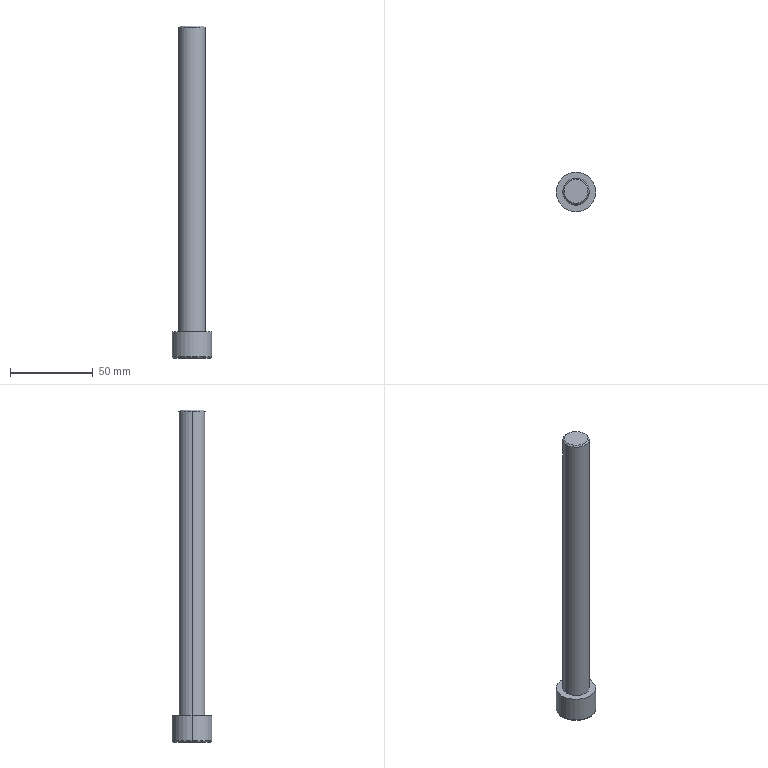Part | Creo | 1 solid | 20 faces | box 24 x 24 x 201 mm | volume 43051 mm3 | plane 10 | cylinder 4 | torus 4 | cone 2 | commonest cylinder face diameters 16 x2 24 x2
STEP:
#1=CARTESIAN_POINT('',(0.,0.,0.));
#2=DIRECTION('',(0.,0.,1.));
#3=DIRECTION('',(1.,0.,0.));
#4=AXIS2_PLACEMENT_3D('',#1,#2,#3);
#5=CARTESIAN_POINT('',(-153.,0.,-293.2));
#6=VERTEX_POINT('',#5);
#7=CARTESIAN_POINT('',(-177.,0.,-293.2));
#8=VERTEX_POINT('',#7);
#9=CARTESIAN_POINT('',(-165.,0.,-293.2));
#10=DIRECTION('',(0.,0.,-1.));
#11=DIRECTION('',(1.,0.,0.));
#12=AXIS2_PLACEMENT_3D('',#9,#10,#11);
#13=CIRCLE('',#12,12.);
#14=EDGE_CURVE('',#6,#8,#13,.T.);
#15=ORIENTED_EDGE('',*,*,#14,.T.);
#16=CARTESIAN_POINT('',(-177.,0.,-278.));
#17=VERTEX_POINT('',#16);
#18=CARTESIAN_POINT('',(-177.,0.,-278.));
#19=DIRECTION('',(0.,0.,-1.));
#20=VECTOR('',#19,15.2);
#21=LINE('',#18,#20);
#22=EDGE_CURVE('',#17,#8,#21,.T.);
#23=ORIENTED_EDGE('',*,*,#22,.F.);
#24=CARTESIAN_POINT('',(-153.,0.,-278.));
#25=VERTEX_POINT('',#24);
#26=CARTESIAN_POINT('',(-165.,0.,-278.));
#27=DIRECTION('',(0.,0.,1.));
#28=DIRECTION('',(-1.,0.,0.));
#29=AXIS2_PLACEMENT_3D('',#26,#27,#28);
#30=CIRCLE('',#29,12.);
#31=EDGE_CURVE('',#17,#25,#30,.T.);
#32=ORIENTED_EDGE('',*,*,#31,.T.);
#33=CARTESIAN_POINT('',(-153.,0.,-278.));
#34=DIRECTION('',(0.,0.,-1.));
#35=VECTOR('',#34,15.2);
#36=LINE('',#33,#35);
#37=EDGE_CURVE('',#25,#6,#36,.T.);
#38=ORIENTED_EDGE('',*,*,#37,.T.);
#39=EDGE_LOOP('',(#15,#23,#32,#38));
#40=FACE_OUTER_BOUND('',#39,.F.);
#41=CARTESIAN_POINT('',(-165.,0.,-278.));
#42=DIRECTION('',(0.,0.,-1.));
#43=DIRECTION('',(1.,0.,0.));
#44=AXIS2_PLACEMENT_3D('',#41,#42,#43);
#45=CYLINDRICAL_SURFACE('',#44,12.);
#46=ADVANCED_FACE('',(#40),#45,.T.);
#47=ORIENTED_EDGE('',*,*,#14,.F.);
#48=CARTESIAN_POINT('',(-153.234,0.,-293.766));
#49=VERTEX_POINT('',#48);
#50=CARTESIAN_POINT('',(-153.8,0.,-293.2));
#51=DIRECTION('',(0.,1.,0.));
#52=DIRECTION('',(1.,0.,0.));
#53=AXIS2_PLACEMENT_3D('',#50,#51,#52);
#54=CIRCLE('',#53,0.8);
#55=EDGE_CURVE('',#6,#49,#54,.T.);
#56=ORIENTED_EDGE('',*,*,#55,.T.);
#57=CARTESIAN_POINT('',(-176.766,0.,-293.766));
#58=VERTEX_POINT('',#57);
#59=CARTESIAN_POINT('',(-165.,0.,-293.766));
#60=DIRECTION('',(0.,0.,-1.));
#61=DIRECTION('',(1.,0.,0.));
#62=AXIS2_PLACEMENT_3D('',#59,#60,#61);
#63=CIRCLE('',#62,11.766);
#64=EDGE_CURVE('',#49,#58,#63,.T.);
#65=ORIENTED_EDGE('',*,*,#64,.T.);
#66=CARTESIAN_POINT('',(-176.2,0.,-293.2));
#67=DIRECTION('',(0.,-1.,0.));
#68=DIRECTION('',(-1.,0.,0.));
#69=AXIS2_PLACEMENT_3D('',#66,#67,#68);
#70=CIRCLE('',#69,0.8);
#71=EDGE_CURVE('',#8,#58,#70,.T.);
#72=ORIENTED_EDGE('',*,*,#71,.F.);
#73=EDGE_LOOP('',(#47,#56,#65,#72));
#74=FACE_OUTER_BOUND('',#73,.F.);
#75=CARTESIAN_POINT('',(-165.,0.,-293.2));
#76=DIRECTION('',(0.,0.,-1.));
#77=DIRECTION('',(1.,0.,0.));
#78=AXIS2_PLACEMENT_3D('',#75,#76,#77);
#79=TOROIDAL_SURFACE('',#78,11.2,0.8);
#80=ADVANCED_FACE('',(#74),#79,.T.);
#81=CARTESIAN_POINT('',(-165.,0.,-293.2));
#82=DIRECTION('',(0.,0.,-1.));
#83=DIRECTION('',(-1.,0.,0.));
#84=AXIS2_PLACEMENT_3D('',#81,#82,#83);
#85=CIRCLE('',#84,12.);
#86=EDGE_CURVE('',#8,#6,#85,.T.);
#87=ORIENTED_EDGE('',*,*,#86,.F.);
#88=ORIENTED_EDGE('',*,*,#71,.T.);
#89=CARTESIAN_POINT('',(-165.,0.,-293.766));
#90=DIRECTION('',(0.,0.,-1.));
#91=DIRECTION('',(-1.,0.,0.));
#92=AXIS2_PLACEMENT_3D('',#89,#90,#91);
#93=CIRCLE('',#92,11.766);
#94=EDGE_CURVE('',#58,#49,#93,.T.);
#95=ORIENTED_EDGE('',*,*,#94,.T.);
#96=ORIENTED_EDGE('',*,*,#55,.F.);
#97=EDGE_LOOP('',(#87,#88,#95,#96));
#98=FACE_OUTER_BOUND('',#97,.F.);
#99=CARTESIAN_POINT('',(-165.,0.,-293.2));
#100=DIRECTION('',(0.,0.,-1.));
#101=DIRECTION('',(1.,0.,0.));
#102=AXIS2_PLACEMENT_3D('',#99,#100,#101);
#103=TOROIDAL_SURFACE('',#102,11.2,0.8);
#104=ADVANCED_FACE('',(#98),#103,.T.);
#105=ORIENTED_EDGE('',*,*,#86,.T.);
#106=ORIENTED_EDGE('',*,*,#37,.F.);
#107=CARTESIAN_POINT('',(-165.,0.,-278.));
#108=DIRECTION('',(0.,0.,1.));
#109=DIRECTION('',(1.,0.,0.));
#110=AXIS2_PLACEMENT_3D('',#107,#108,#109);
#111=CIRCLE('',#110,12.);
#112=EDGE_CURVE('',#25,#17,#111,.T.);
#113=ORIENTED_EDGE('',*,*,#112,.T.);
#114=ORIENTED_EDGE('',*,*,#22,.T.);
#115=EDGE_LOOP('',(#105,#106,#113,#114));
#116=FACE_OUTER_BOUND('',#115,.F.);
#117=CARTESIAN_POINT('',(-165.,0.,-278.));
#118=DIRECTION('',(0.,0.,-1.));
#119=DIRECTION('',(1.,0.,0.));
#120=AXIS2_PLACEMENT_3D('',#117,#118,#119);
#121=CYLINDRICAL_SURFACE('',#120,12.);
#122=ADVANCED_FACE('',(#116),#121,.T.);
#123=ORIENTED_EDGE('',*,*,#31,.F.);
#124=ORIENTED_EDGE('',*,*,#112,.F.);
#125=EDGE_LOOP('',(#123,#124));
#126=FACE_OUTER_BOUND('',#125,.F.);
#127=CARTESIAN_POINT('',(-157.,0.,-278.));
#128=VERTEX_POINT('',#127);
#129=CARTESIAN_POINT('',(-173.,0.,-278.));
#130=VERTEX_POINT('',#129);
#131=CARTESIAN_POINT('',(-165.,0.,-278.));
#132=DIRECTION('',(0.,0.,-1.));
#133=DIRECTION('',(1.,0.,0.));
#134=AXIS2_PLACEMENT_3D('',#131,#132,#133);
#135=CIRCLE('',#134,8.);
#136=EDGE_CURVE('',#128,#130,#135,.T.);
#137=ORIENTED_EDGE('',*,*,#136,.F.);
#138=CARTESIAN_POINT('',(-165.,0.,-278.));
#139=DIRECTION('',(0.,0.,-1.));
#140=DIRECTION('',(-1.,0.,0.));
#141=AXIS2_PLACEMENT_3D('',#138,#139,#140);
#142=CIRCLE('',#141,8.);
#143=EDGE_CURVE('',#130,#128,#142,.T.);
#144=ORIENTED_EDGE('',*,*,#143,.F.);
#145=EDGE_LOOP('',(#137,#144));
#146=FACE_BOUND('',#145,.F.);
#147=CARTESIAN_POINT('',(-165.,0.,-278.));
#148=DIRECTION('',(0.,0.,-1.));
#149=DIRECTION('',(1.,0.,0.));
#150=AXIS2_PLACEMENT_3D('',#147,#148,#149);
#151=PLANE('',#150);
#152=ADVANCED_FACE('',(#126,#146),#151,.F.);
#153=CARTESIAN_POINT('',(-173.,0.,-93.8));
#154=VERTEX_POINT('',#153);
#155=CARTESIAN_POINT('',(-157.,0.,-93.8));
#156=VERTEX_POINT('',#155);
#157=CARTESIAN_POINT('',(-165.,0.,-93.8));
#158=DIRECTION('',(0.,0.,1.));
#159=DIRECTION('',(-1.,0.,0.));
#160=AXIS2_PLACEMENT_3D('',#157,#158,#159);
#161=CIRCLE('',#160,8.);
#162=EDGE_CURVE('',#154,#156,#161,.T.);
#163=ORIENTED_EDGE('',*,*,#162,.T.);
#164=CARTESIAN_POINT('',(-157.,0.,-278.));
#165=DIRECTION('',(0.,0.,1.));
#166=VECTOR('',#165,184.2);
#167=LINE('',#164,#166);
#168=EDGE_CURVE('',#128,#156,#167,.T.);
#169=ORIENTED_EDGE('',*,*,#168,.F.);
#170=ORIENTED_EDGE('',*,*,#136,.T.);
#171=CARTESIAN_POINT('',(-173.,0.,-278.));
#172=DIRECTION('',(0.,0.,1.));
#173=VECTOR('',#172,184.2);
#174=LINE('',#171,#173);
#175=EDGE_CURVE('',#130,#154,#174,.T.);
#176=ORIENTED_EDGE('',*,*,#175,.T.);
#177=EDGE_LOOP('',(#163,#169,#170,#176));
#178=FACE_OUTER_BOUND('',#177,.F.);
#179=CARTESIAN_POINT('',(-165.,0.,-278.));
#180=DIRECTION('',(0.,0.,1.));
#181=DIRECTION('',(-1.,0.,0.));
#182=AXIS2_PLACEMENT_3D('',#179,#180,#181);
#183=CYLINDRICAL_SURFACE('',#182,8.);
#184=ADVANCED_FACE('',(#178),#183,.T.);
#185=ORIENTED_EDGE('',*,*,#162,.F.);
#186=CARTESIAN_POINT('',(-172.2,0.,-93.));
#187=VERTEX_POINT('',#186);
#188=CARTESIAN_POINT('',(-172.2,0.,-93.));
#189=DIRECTION('',(-0.7071,0.,-0.7071));
#190=VECTOR('',#189,1.131);
#191=LINE('',#188,#190);
#192=EDGE_CURVE('',#187,#154,#191,.T.);
#193=ORIENTED_EDGE('',*,*,#192,.F.);
#194=CARTESIAN_POINT('',(-157.8,0.,-93.));
#195=VERTEX_POINT('',#194);
#196=CARTESIAN_POINT('',(-165.,0.,-93.));
#197=DIRECTION('',(0.,0.,1.));
#198=DIRECTION('',(-1.,0.,0.));
#199=AXIS2_PLACEMENT_3D('',#196,#197,#198);
#200=CIRCLE('',#199,7.2);
#201=EDGE_CURVE('',#187,#195,#200,.T.);
#202=ORIENTED_EDGE('',*,*,#201,.T.);
#203=CARTESIAN_POINT('',(-157.8,0.,-93.));
#204=DIRECTION('',(0.7071,0.,-0.7071));
#205=VECTOR('',#204,1.131);
#206=LINE('',#203,#205);
#207=EDGE_CURVE('',#195,#156,#206,.T.);
#208=ORIENTED_EDGE('',*,*,#207,.T.);
#209=EDGE_LOOP('',(#185,#193,#202,#208));
#210=FACE_OUTER_BOUND('',#209,.F.);
#211=CARTESIAN_POINT('',(-165.,0.,-93.4));
#212=DIRECTION('',(0.,0.,-1.));
#213=DIRECTION('',(1.,0.,0.));
#214=AXIS2_PLACEMENT_3D('',#211,#212,#213);
#215=CONICAL_SURFACE('',#214,7.6,45.);
#216=ADVANCED_FACE('',(#210),#215,.T.);
#217=CARTESIAN_POINT('',(-165.,0.,-93.8));
#218=DIRECTION('',(0.,0.,1.));
#219=DIRECTION('',(1.,0.,0.));
#220=AXIS2_PLACEMENT_3D('',#217,#218,#219);
#221=CIRCLE('',#220,8.);
#222=EDGE_CURVE('',#156,#154,#221,.T.);
#223=ORIENTED_EDGE('',*,*,#222,.F.);
#224=ORIENTED_EDGE('',*,*,#207,.F.);
#225=CARTESIAN_POINT('',(-165.,0.,-93.));
#226=DIRECTION('',(0.,0.,1.));
#227=DIRECTION('',(1.,0.,0.));
#228=AXIS2_PLACEMENT_3D('',#225,#226,#227);
#229=CIRCLE('',#228,7.2);
#230=EDGE_CURVE('',#195,#187,#229,.T.);
#231=ORIENTED_EDGE('',*,*,#230,.T.);
#232=ORIENTED_EDGE('',*,*,#192,.T.);
#233=EDGE_LOOP('',(#223,#224,#231,#232));
#234=FACE_OUTER_BOUND('',#233,.F.);
#235=CARTESIAN_POINT('',(-165.,0.,-93.4));
#236=DIRECTION('',(0.,0.,-1.));
#237=DIRECTION('',(1.,0.,0.));
#238=AXIS2_PLACEMENT_3D('',#235,#236,#237);
#239=CONICAL_SURFACE('',#238,7.6,45.);
#240=ADVANCED_FACE('',(#234),#239,.T.);
#241=ORIENTED_EDGE('',*,*,#222,.T.);
#242=ORIENTED_EDGE('',*,*,#175,.F.);
#243=ORIENTED_EDGE('',*,*,#143,.T.);
#244=ORIENTED_EDGE('',*,*,#168,.T.);
#245=EDGE_LOOP('',(#241,#242,#243,#244));
#246=FACE_OUTER_BOUND('',#245,.F.);
#247=CARTESIAN_POINT('',(-165.,0.,-278.));
#248=DIRECTION('',(0.,0.,1.));
#249=DIRECTION('',(-1.,0.,0.));
#250=AXIS2_PLACEMENT_3D('',#247,#248,#249);
#251=CYLINDRICAL_SURFACE('',#250,8.);
#252=ADVANCED_FACE('',(#246),#251,.T.);
#253=ORIENTED_EDGE('',*,*,#230,.F.);
#254=ORIENTED_EDGE('',*,*,#201,.F.);
#255=EDGE_LOOP('',(#253,#254));
#256=FACE_OUTER_BOUND('',#255,.F.);
#257=CARTESIAN_POINT('',(-165.,0.,-93.));
#258=DIRECTION('',(0.,0.,1.));
#259=DIRECTION('',(-1.,0.,0.));
#260=AXIS2_PLACEMENT_3D('',#257,#258,#259);
#261=PLANE('',#260);
#262=ADVANCED_FACE('',(#256),#261,.T.);
#263=CARTESIAN_POINT('',(-176.2,0.,-294.));
#264=VERTEX_POINT('',#263);
#265=CARTESIAN_POINT('',(-153.8,0.,-294.));
#266=VERTEX_POINT('',#265);
#267=CARTESIAN_POINT('',(-165.,0.,-294.));
#268=DIRECTION('',(0.,0.,-1.));
#269=DIRECTION('',(-1.,0.,0.));
#270=AXIS2_PLACEMENT_3D('',#267,#268,#269);
#271=CIRCLE('',#270,11.2);
#272=EDGE_CURVE('',#264,#266,#271,.T.);
#273=ORIENTED_EDGE('',*,*,#272,.T.);
#274=CARTESIAN_POINT('',(-153.8,0.,-293.2));
#275=DIRECTION('',(0.,1.,0.));
#276=DIRECTION('',(0.7071,0.,-0.7071));
#277=AXIS2_PLACEMENT_3D('',#274,#275,#276);
#278=CIRCLE('',#277,0.8);
#279=EDGE_CURVE('',#49,#266,#278,.T.);
#280=ORIENTED_EDGE('',*,*,#279,.F.);
#281=ORIENTED_EDGE('',*,*,#94,.F.);
#282=CARTESIAN_POINT('',(-176.2,0.,-293.2));
#283=DIRECTION('',(0.,-1.,0.));
#284=DIRECTION('',(-0.7071,0.,-0.7071));
#285=AXIS2_PLACEMENT_3D('',#282,#283,#284);
#286=CIRCLE('',#285,0.8);
#287=EDGE_CURVE('',#58,#264,#286,.T.);
#288=ORIENTED_EDGE('',*,*,#287,.T.);
#289=EDGE_LOOP('',(#273,#280,#281,#288));
#290=FACE_OUTER_BOUND('',#289,.F.);
#291=CARTESIAN_POINT('',(-165.,0.,-293.2));
#292=DIRECTION('',(0.,0.,-1.));
#293=DIRECTION('',(1.,0.,0.));
#294=AXIS2_PLACEMENT_3D('',#291,#292,#293);
#295=TOROIDAL_SURFACE('',#294,11.2,0.8);
#296=ADVANCED_FACE('',(#290),#295,.T.);
#297=ORIENTED_EDGE('',*,*,#272,.F.);
#298=CARTESIAN_POINT('',(-165.,0.,-294.));
#299=DIRECTION('',(0.,0.,-1.));
#300=DIRECTION('',(1.,0.,0.));
#301=AXIS2_PLACEMENT_3D('',#298,#299,#300);
#302=CIRCLE('',#301,11.2);
#303=EDGE_CURVE('',#266,#264,#302,.T.);
#304=ORIENTED_EDGE('',*,*,#303,.F.);
#305=EDGE_LOOP('',(#297,#304));
#306=FACE_OUTER_BOUND('',#305,.F.);
#307=CARTESIAN_POINT('',(-169.041,-7.,-294.));
#308=VERTEX_POINT('',#307);
#309=CARTESIAN_POINT('',(-160.959,-7.,-294.));
#310=VERTEX_POINT('',#309);
#311=CARTESIAN_POINT('',(-169.041,-7.,-294.));
#312=DIRECTION('',(1.,0.,0.));
#313=VECTOR('',#312,8.083);
#314=LINE('',#311,#313);
#315=EDGE_CURVE('',#308,#310,#314,.T.);
#316=ORIENTED_EDGE('',*,*,#315,.F.);
#317=CARTESIAN_POINT('',(-173.083,0.,-294.));
#318=VERTEX_POINT('',#317);
#319=CARTESIAN_POINT('',(-173.083,0.,-294.));
#320=DIRECTION('',(0.5,-0.866,0.));
#321=VECTOR('',#320,8.083);
#322=LINE('',#319,#321);
#323=EDGE_CURVE('',#318,#308,#322,.T.);
#324=ORIENTED_EDGE('',*,*,#323,.F.);
#325=CARTESIAN_POINT('',(-169.041,7.,-294.));
#326=VERTEX_POINT('',#325);
#327=CARTESIAN_POINT('',(-169.041,7.,-294.));
#328=DIRECTION('',(-0.5,-0.866,0.));
#329=VECTOR('',#328,8.083);
#330=LINE('',#327,#329);
#331=EDGE_CURVE('',#326,#318,#330,.T.);
#332=ORIENTED_EDGE('',*,*,#331,.F.);
#333=CARTESIAN_POINT('',(-160.959,7.,-294.));
#334=VERTEX_POINT('',#333);
#335=CARTESIAN_POINT('',(-160.959,7.,-294.));
#336=DIRECTION('',(-1.,0.,0.));
#337=VECTOR('',#336,8.083);
#338=LINE('',#335,#337);
#339=EDGE_CURVE('',#334,#326,#338,.T.);
#340=ORIENTED_EDGE('',*,*,#339,.F.);
#341=CARTESIAN_POINT('',(-156.917,0.,-294.));
#342=VERTEX_POINT('',#341);
#343=CARTESIAN_POINT('',(-156.917,0.,-294.));
#344=DIRECTION('',(-0.5,0.866,0.));
#345=VECTOR('',#344,8.083);
#346=LINE('',#343,#345);
#347=EDGE_CURVE('',#342,#334,#346,.T.);
#348=ORIENTED_EDGE('',*,*,#347,.F.);
#349=CARTESIAN_POINT('',(-160.959,-7.,-294.));
#350=DIRECTION('',(0.5,0.866,0.));
#351=VECTOR('',#350,8.083);
#352=LINE('',#349,#351);
#353=EDGE_CURVE('',#310,#342,#352,.T.);
#354=ORIENTED_EDGE('',*,*,#353,.F.);
#355=EDGE_LOOP('',(#316,#324,#332,#340,#348,#354));
#356=FACE_BOUND('',#355,.F.);
#357=CARTESIAN_POINT('',(-165.,0.,-294.));
#358=DIRECTION('',(0.,0.,-1.));
#359=DIRECTION('',(1.,0.,0.));
#360=AXIS2_PLACEMENT_3D('',#357,#358,#359);
#361=PLANE('',#360);
#362=ADVANCED_FACE('',(#306,#356),#361,.T.);
#363=ORIENTED_EDGE('',*,*,#303,.T.);
#364=ORIENTED_EDGE('',*,*,#287,.F.);
#365=ORIENTED_EDGE('',*,*,#64,.F.);
#366=ORIENTED_EDGE('',*,*,#279,.T.);
#367=EDGE_LOOP('',(#363,#364,#365,#366));
#368=FACE_OUTER_BOUND('',#367,.F.);
#369=CARTESIAN_POINT('',(-165.,0.,-293.2));
#370=DIRECTION('',(0.,0.,-1.));
#371=DIRECTION('',(1.,0.,0.));
#372=AXIS2_PLACEMENT_3D('',#369,#370,#371);
#373=TOROIDAL_SURFACE('',#372,11.2,0.8);
#374=ADVANCED_FACE('',(#368),#373,.T.);
#375=ORIENTED_EDGE('',*,*,#315,.T.);
#376=CARTESIAN_POINT('',(-160.959,-7.,-286.));
#377=VERTEX_POINT('',#376);
#378=CARTESIAN_POINT('',(-160.959,-7.,-294.));
#379=DIRECTION('',(0.,0.,1.));
#380=VECTOR('',#379,8.);
#381=LINE('',#378,#380);
#382=EDGE_CURVE('',#310,#377,#381,.T.);
#383=ORIENTED_EDGE('',*,*,#382,.T.);
#384=CARTESIAN_POINT('',(-169.041,-7.,-286.));
#385=VERTEX_POINT('',#384);
#386=CARTESIAN_POINT('',(-169.041,-7.,-286.));
#387=DIRECTION('',(1.,0.,0.));
#388=VECTOR('',#387,8.083);
#389=LINE('',#386,#388);
#390=EDGE_CURVE('',#385,#377,#389,.T.);
#391=ORIENTED_EDGE('',*,*,#390,.F.);
#392=CARTESIAN_POINT('',(-169.041,-7.,-294.));
#393=DIRECTION('',(0.,0.,1.));
#394=VECTOR('',#393,8.);
#395=LINE('',#392,#394);
#396=EDGE_CURVE('',#308,#385,#395,.T.);
#397=ORIENTED_EDGE('',*,*,#396,.F.);
#398=EDGE_LOOP('',(#375,#383,#391,#397));
#399=FACE_OUTER_BOUND('',#398,.F.);
#400=CARTESIAN_POINT('',(-160.959,-7.,-286.));
#401=DIRECTION('',(0.,-1.,0.));
#402=DIRECTION('',(1.,0.,0.));
#403=AXIS2_PLACEMENT_3D('',#400,#401,#402);
#404=PLANE('',#403);
#405=ADVANCED_FACE('',(#399),#404,.F.);
#406=ORIENTED_EDGE('',*,*,#353,.T.);
#407=CARTESIAN_POINT('',(-156.917,0.,-286.));
#408=VERTEX_POINT('',#407);
#409=CARTESIAN_POINT('',(-156.917,0.,-294.));
#410=DIRECTION('',(0.,0.,1.));
#411=VECTOR('',#410,8.);
#412=LINE('',#409,#411);
#413=EDGE_CURVE('',#342,#408,#412,.T.);
#414=ORIENTED_EDGE('',*,*,#413,.T.);
#415=CARTESIAN_POINT('',(-156.917,0.,-286.));
#416=DIRECTION('',(-0.5,-0.866,0.));
#417=VECTOR('',#416,8.083);
#418=LINE('',#415,#417);
#419=EDGE_CURVE('',#408,#377,#418,.T.);
#420=ORIENTED_EDGE('',*,*,#419,.T.);
#421=ORIENTED_EDGE('',*,*,#382,.F.);
#422=EDGE_LOOP('',(#406,#414,#420,#421));
#423=FACE_OUTER_BOUND('',#422,.F.);
#424=CARTESIAN_POINT('',(-156.917,0.,-286.));
#425=DIRECTION('',(0.866,-0.5,0.));
#426=DIRECTION('',(0.5,0.866,0.));
#427=AXIS2_PLACEMENT_3D('',#424,#425,#426);
#428=PLANE('',#427);
#429=ADVANCED_FACE('',(#423),#428,.F.);
#430=ORIENTED_EDGE('',*,*,#347,.T.);
#431=CARTESIAN_POINT('',(-160.959,7.,-286.));
#432=VERTEX_POINT('',#431);
#433=CARTESIAN_POINT('',(-160.959,7.,-294.));
#434=DIRECTION('',(0.,0.,1.));
#435=VECTOR('',#434,8.);
#436=LINE('',#433,#435);
#437=EDGE_CURVE('',#334,#432,#436,.T.);
#438=ORIENTED_EDGE('',*,*,#437,.T.);
#439=CARTESIAN_POINT('',(-160.959,7.,-286.));
#440=DIRECTION('',(0.5,-0.866,0.));
#441=VECTOR('',#440,8.083);
#442=LINE('',#439,#441);
#443=EDGE_CURVE('',#432,#408,#442,.T.);
#444=ORIENTED_EDGE('',*,*,#443,.T.);
#445=ORIENTED_EDGE('',*,*,#413,.F.);
#446=EDGE_LOOP('',(#430,#438,#444,#445));
#447=FACE_OUTER_BOUND('',#446,.F.);
#448=CARTESIAN_POINT('',(-160.959,7.,-286.));
#449=DIRECTION('',(0.866,0.5,0.));
#450=DIRECTION('',(-0.5,0.866,0.));
#451=AXIS2_PLACEMENT_3D('',#448,#449,#450);
#452=PLANE('',#451);
#453=ADVANCED_FACE('',(#447),#452,.F.);
#454=ORIENTED_EDGE('',*,*,#339,.T.);
#455=CARTESIAN_POINT('',(-169.041,7.,-286.));
#456=VERTEX_POINT('',#455);
#457=CARTESIAN_POINT('',(-169.041,7.,-294.));
#458=DIRECTION('',(0.,0.,1.));
#459=VECTOR('',#458,8.);
#460=LINE('',#457,#459);
#461=EDGE_CURVE('',#326,#456,#460,.T.);
#462=ORIENTED_EDGE('',*,*,#461,.T.);
#463=CARTESIAN_POINT('',(-160.959,7.,-286.));
#464=DIRECTION('',(-1.,0.,0.));
#465=VECTOR('',#464,8.083);
#466=LINE('',#463,#465);
#467=EDGE_CURVE('',#432,#456,#466,.T.);
#468=ORIENTED_EDGE('',*,*,#467,.F.);
#469=ORIENTED_EDGE('',*,*,#437,.F.);
#470=EDGE_LOOP('',(#454,#462,#468,#469));
#471=FACE_OUTER_BOUND('',#470,.F.);
#472=CARTESIAN_POINT('',(-169.041,7.,-286.));
#473=DIRECTION('',(0.,1.,0.));
#474=DIRECTION('',(-1.,0.,0.));
#475=AXIS2_PLACEMENT_3D('',#472,#473,#474);
#476=PLANE('',#475);
#477=ADVANCED_FACE('',(#471),#476,.F.);
#478=ORIENTED_EDGE('',*,*,#331,.T.);
#479=CARTESIAN_POINT('',(-173.083,0.,-286.));
#480=VERTEX_POINT('',#479);
#481=CARTESIAN_POINT('',(-173.083,0.,-294.));
#482=DIRECTION('',(0.,0.,1.));
#483=VECTOR('',#482,8.);
#484=LINE('',#481,#483);
#485=EDGE_CURVE('',#318,#480,#484,.T.);
#486=ORIENTED_EDGE('',*,*,#485,.T.);
#487=CARTESIAN_POINT('',(-173.083,0.,-286.));
#488=DIRECTION('',(0.5,0.866,0.));
#489=VECTOR('',#488,8.083);
#490=LINE('',#487,#489);
#491=EDGE_CURVE('',#480,#456,#490,.T.);
#492=ORIENTED_EDGE('',*,*,#491,.T.);
#493=ORIENTED_EDGE('',*,*,#461,.F.);
#494=EDGE_LOOP('',(#478,#486,#492,#493));
#495=FACE_OUTER_BOUND('',#494,.F.);
#496=CARTESIAN_POINT('',(-173.083,0.,-286.));
#497=DIRECTION('',(-0.866,0.5,0.));
#498=DIRECTION('',(-0.5,-0.866,0.));
#499=AXIS2_PLACEMENT_3D('',#496,#497,#498);
#500=PLANE('',#499);
#501=ADVANCED_FACE('',(#495),#500,.F.);
#502=ORIENTED_EDGE('',*,*,#323,.T.);
#503=ORIENTED_EDGE('',*,*,#396,.T.);
#504=CARTESIAN_POINT('',(-169.041,-7.,-286.));
#505=DIRECTION('',(-0.5,0.866,0.));
#506=VECTOR('',#505,8.083);
#507=LINE('',#504,#506);
#508=EDGE_CURVE('',#385,#480,#507,.T.);
#509=ORIENTED_EDGE('',*,*,#508,.T.);
#510=ORIENTED_EDGE('',*,*,#485,.F.);
#511=EDGE_LOOP('',(#502,#503,#509,#510));
#512=FACE_OUTER_BOUND('',#511,.F.);
#513=CARTESIAN_POINT('',(-169.041,-7.,-286.));
#514=DIRECTION('',(-0.866,-0.5,0.));
#515=DIRECTION('',(0.5,-0.866,0.));
#516=AXIS2_PLACEMENT_3D('',#513,#514,#515);
#517=PLANE('',#516);
#518=ADVANCED_FACE('',(#512),#517,.F.);
#519=ORIENTED_EDGE('',*,*,#390,.T.);
#520=ORIENTED_EDGE('',*,*,#419,.F.);
#521=ORIENTED_EDGE('',*,*,#443,.F.);
#522=ORIENTED_EDGE('',*,*,#467,.T.);
#523=ORIENTED_EDGE('',*,*,#491,.F.);
#524=ORIENTED_EDGE('',*,*,#508,.F.);
#525=EDGE_LOOP('',(#519,#520,#521,#522,#523,#524));
#526=FACE_OUTER_BOUND('',#525,.F.);
#527=CARTESIAN_POINT('',(-177.124,-7.,-286.));
#528=DIRECTION('',(0.,0.,-1.));
#529=DIRECTION('',(1.,0.,0.));
#530=AXIS2_PLACEMENT_3D('',#527,#528,#529);
#531=PLANE('',#530);
#532=ADVANCED_FACE('',(#526),#531,.T.);
#533=CLOSED_SHELL('',(#46,#80,#104,#122,#152,#184,#216,#240,#252,#262,#296,#362,#374,#405,#429,#453,#477,#501,#518,#532));
#534=MANIFOLD_SOLID_BREP('',#533);
#535=(LENGTH_UNIT()NAMED_UNIT(*)SI_UNIT(.MILLI.,.METRE.));
#536=UNCERTAINTY_MEASURE_WITH_UNIT(LENGTH_MEASURE(0.02038),#535,'','');
#537=(NAMED_UNIT(*)PLANE_ANGLE_UNIT()SI_UNIT($,.RADIAN.));
#538=PLANE_ANGLE_MEASURE_WITH_UNIT(PLANE_ANGLE_MEASURE(0.01745),#537);
#539=(CONVERSION_BASED_UNIT('DEGREE',#538)NAMED_UNIT(*)PLANE_ANGLE_UNIT());
#540=(NAMED_UNIT(*)SI_UNIT($,.STERADIAN.)SOLID_ANGLE_UNIT());
#541=(GEOMETRIC_REPRESENTATION_CONTEXT(3)GLOBAL_UNCERTAINTY_ASSIGNED_CONTEXT((#536))GLOBAL_UNIT_ASSIGNED_CONTEXT((#535,#539,#540))REPRESENTATION_CONTEXT('',''));
#542=ADVANCED_BREP_SHAPE_REPRESENTATION('',(#4,#534),#541);